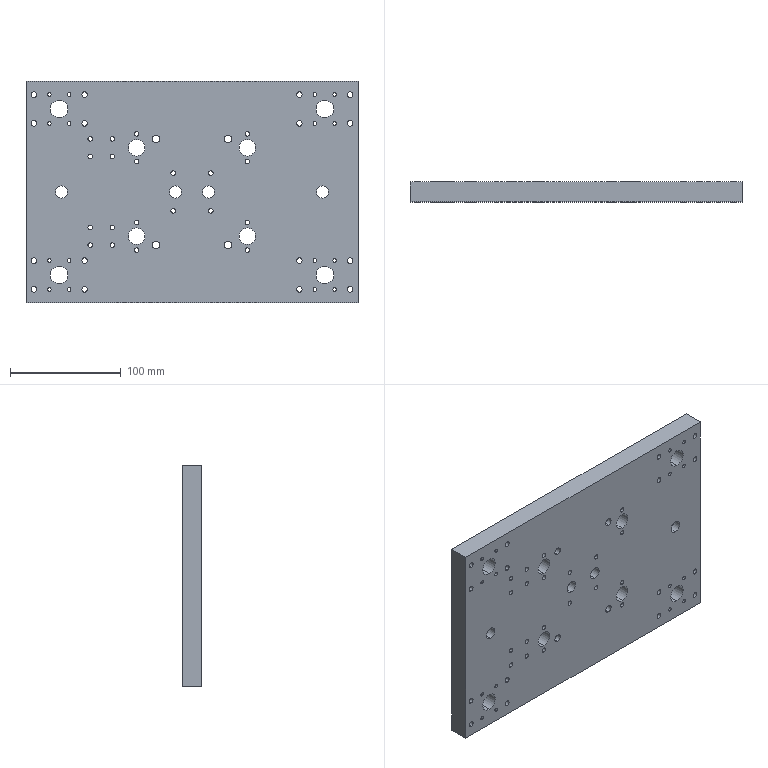Part | STEP file | 1 solid | 162 faces | box 300 x 18 x 200 mm | volume 1023453 mm3 | cylinder 144 | plane 10 | cone 8 | commonest cylinder face diameters 4.2 x40 3.3 x32 5 x32 6.8 x8 11 x8 15 x8